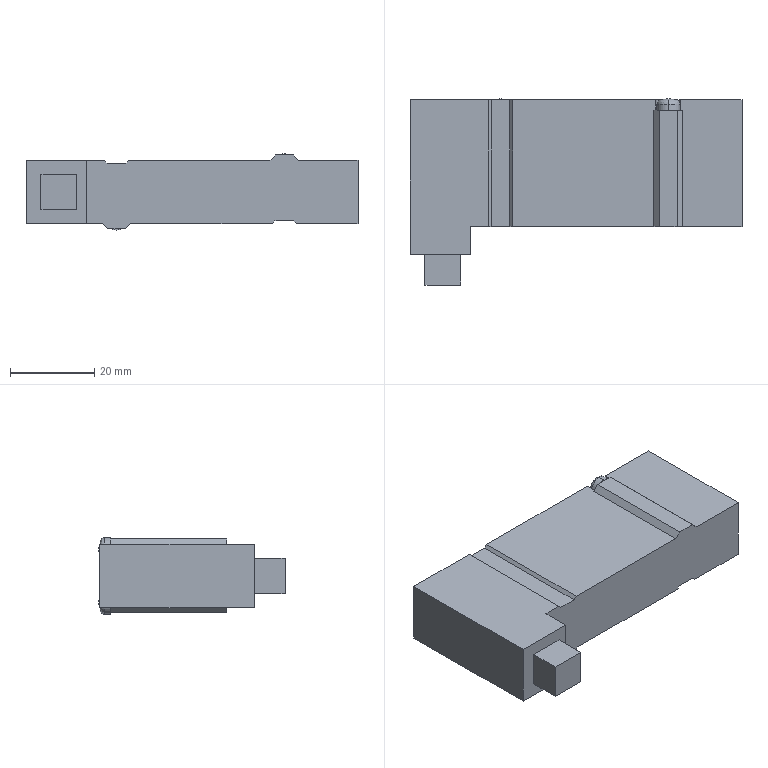Part | SolidWorks | features BaseBody 1 | 1 solid | 76 faces | box 78.8 x 44.194 x 18.1 mm | volume 37684 mm3 | plane 63 | cylinder 7 | spline 6 | commonest cylinder face diameters 5.5 x4 6 x3